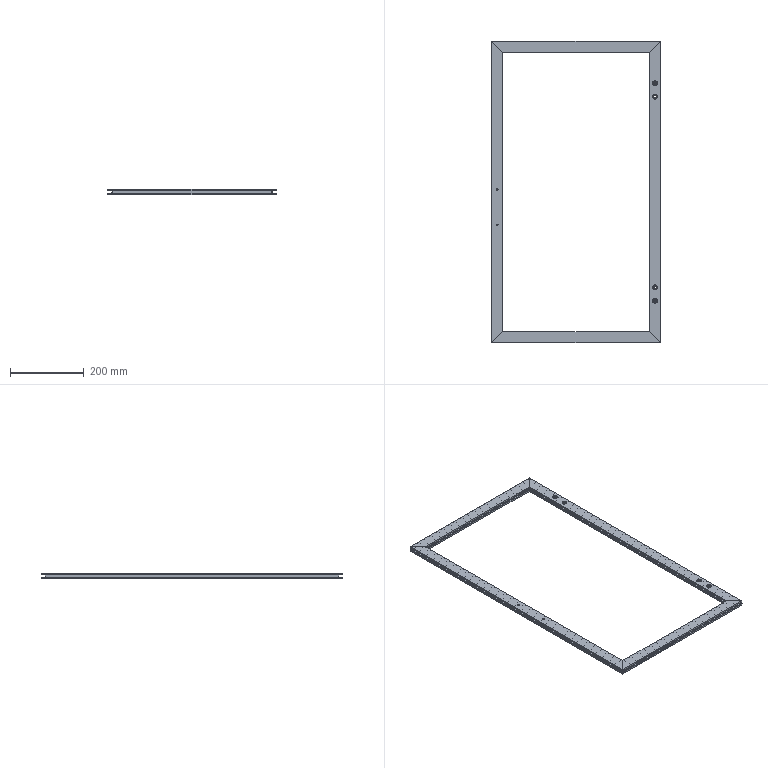Part | STEP file | Cabinet door_Default<machined> | 4 solids | 160 faces | box 457.5 x 818 x 15 mm | volume 630876 mm3 | plane 124 | cylinder 36 | commonest cylinder face diameters 5 x12 4 x8 6.6 x8 13 x8